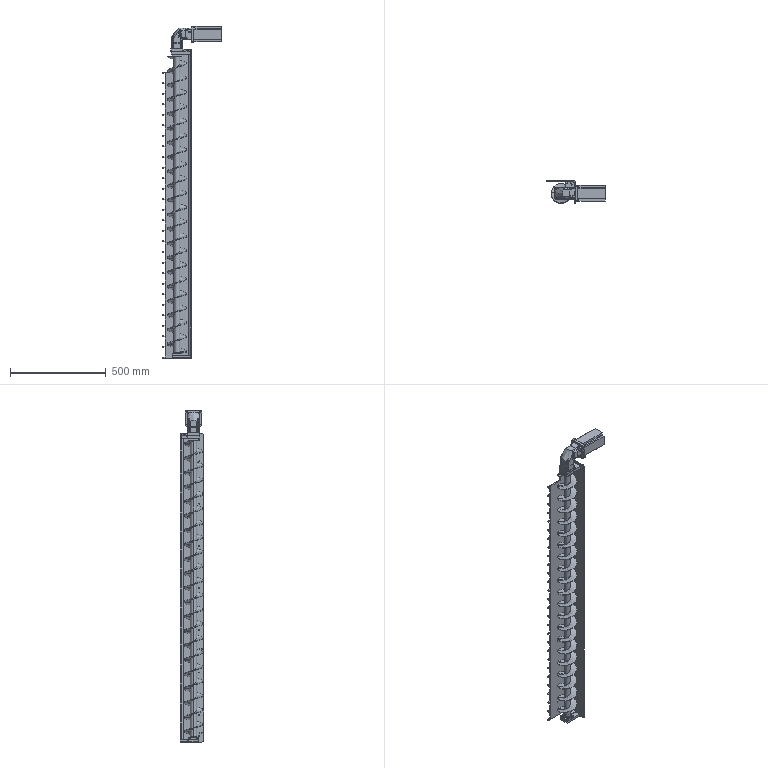Part | SolidWorks | features InContextFeatHolder 2 | 24 solids | 1157 faces | box 307 x 120 x 1730 mm | volume 4796774 mm3 | cylinder 504 | plane 451 | cone 125 | spline 53 | torus 24 | commonest cylinder face diameters 4.2 x96 5.8 x34 5.5 x28 10 x28 69 x26 5 x21